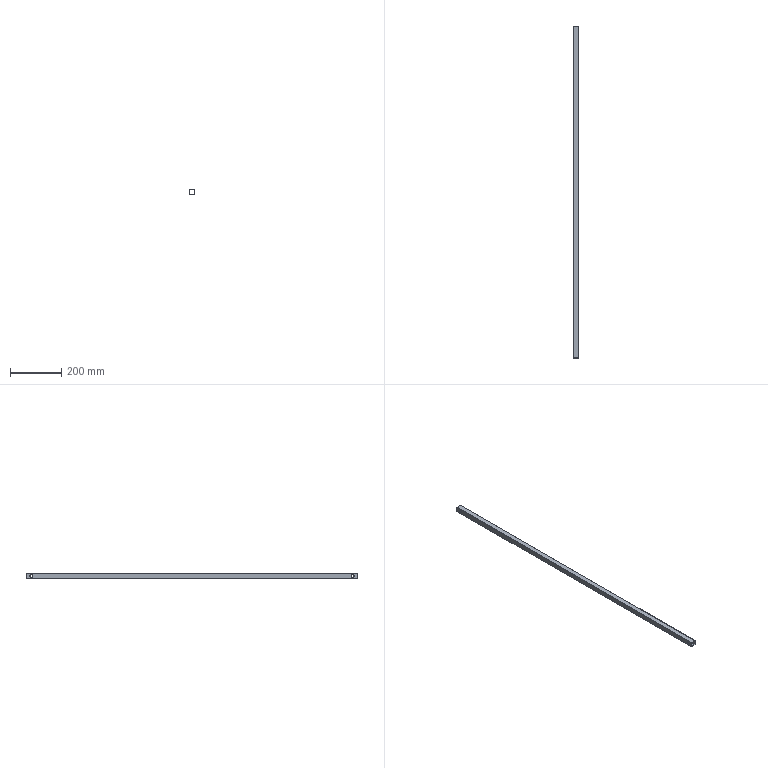Part | SolidWorks | features HoleWzd 1, WeldMemberFeat 1, WeldmentFeature 1 | 1 solid | 18 faces | box 20 x 1300 x 20 mm | volume 98454 mm3 | plane 10 | cylinder 8 | commonest cylinder face diameters 10.5 x8
STEP:
#1=CARTESIAN_POINT('',(-10.,20.,5.25));
#2=VERTEX_POINT('',#1);
#3=CARTESIAN_POINT('',(-10.,20.,-5.25));
#4=VERTEX_POINT('',#3);
#5=CARTESIAN_POINT('',(-10.,20.,0.));
#6=DIRECTION('',(1.,0.,0.));
#7=DIRECTION('',(0.,0.,-1.));
#8=AXIS2_PLACEMENT_3D('',#5,#6,#7);
#9=CIRCLE('',#8,5.25);
#10=EDGE_CURVE('',#2,#4,#9,.T.);
#11=ORIENTED_EDGE('',*,*,#10,.F.);
#12=CARTESIAN_POINT('',(-9.,20.,5.25));
#13=VERTEX_POINT('',#12);
#14=CARTESIAN_POINT('',(10.,20.,5.25));
#15=DIRECTION('',(1.,0.,0.));
#16=VECTOR('',#15,1000.);
#17=LINE('',#14,#16);
#18=EDGE_CURVE('',#2,#13,#17,.T.);
#19=ORIENTED_EDGE('',*,*,#18,.T.);
#20=CARTESIAN_POINT('',(-9.,20.,-5.25));
#21=VERTEX_POINT('',#20);
#22=CARTESIAN_POINT('',(-9.,20.,0.));
#23=DIRECTION('',(1.,0.,0.));
#24=DIRECTION('',(0.,0.,-1.));
#25=AXIS2_PLACEMENT_3D('',#22,#23,#24);
#26=CIRCLE('',#25,5.25);
#27=EDGE_CURVE('',#13,#21,#26,.T.);
#28=ORIENTED_EDGE('',*,*,#27,.T.);
#29=CARTESIAN_POINT('',(10.,20.,-5.25));
#30=DIRECTION('',(1.,0.,0.));
#31=VECTOR('',#30,1000.);
#32=LINE('',#29,#31);
#33=EDGE_CURVE('',#4,#21,#32,.T.);
#34=ORIENTED_EDGE('',*,*,#33,.F.);
#35=EDGE_LOOP('',(#11,#19,#28,#34));
#36=FACE_OUTER_BOUND('',#35,.T.);
#37=CARTESIAN_POINT('',(10.,20.,0.));
#38=DIRECTION('',(1.,0.,0.));
#39=DIRECTION('',(0.,0.,-1.));
#40=AXIS2_PLACEMENT_3D('',#37,#38,#39);
#41=CYLINDRICAL_SURFACE('',#40,5.25);
#42=ADVANCED_FACE('',(#36),#41,.F.);
#43=CARTESIAN_POINT('',(9.,20.,-5.25));
#44=VERTEX_POINT('',#43);
#45=CARTESIAN_POINT('',(9.,20.,5.25));
#46=VERTEX_POINT('',#45);
#47=CARTESIAN_POINT('',(9.,20.,0.));
#48=DIRECTION('',(-1.,0.,0.));
#49=DIRECTION('',(0.,0.,1.));
#50=AXIS2_PLACEMENT_3D('',#47,#48,#49);
#51=CIRCLE('',#50,5.25);
#52=EDGE_CURVE('',#44,#46,#51,.T.);
#53=ORIENTED_EDGE('',*,*,#52,.T.);
#54=CARTESIAN_POINT('',(10.,20.,5.25));
#55=VERTEX_POINT('',#54);
#56=CARTESIAN_POINT('',(10.,20.,5.25));
#57=DIRECTION('',(1.,0.,0.));
#58=VECTOR('',#57,1000.);
#59=LINE('',#56,#58);
#60=EDGE_CURVE('',#46,#55,#59,.T.);
#61=ORIENTED_EDGE('',*,*,#60,.T.);
#62=CARTESIAN_POINT('',(10.,20.,-5.25));
#63=VERTEX_POINT('',#62);
#64=CARTESIAN_POINT('',(10.,20.,0.));
#65=DIRECTION('',(1.,0.,0.));
#66=DIRECTION('',(0.,0.,-1.));
#67=AXIS2_PLACEMENT_3D('',#64,#65,#66);
#68=CIRCLE('',#67,5.25);
#69=EDGE_CURVE('',#55,#63,#68,.T.);
#70=ORIENTED_EDGE('',*,*,#69,.T.);
#71=CARTESIAN_POINT('',(10.,20.,-5.25));
#72=DIRECTION('',(1.,0.,0.));
#73=VECTOR('',#72,1000.);
#74=LINE('',#71,#73);
#75=EDGE_CURVE('',#44,#63,#74,.T.);
#76=ORIENTED_EDGE('',*,*,#75,.F.);
#77=EDGE_LOOP('',(#53,#61,#70,#76));
#78=FACE_OUTER_BOUND('',#77,.T.);
#79=CARTESIAN_POINT('',(10.,20.,0.));
#80=DIRECTION('',(1.,0.,0.));
#81=DIRECTION('',(0.,0.,-1.));
#82=AXIS2_PLACEMENT_3D('',#79,#80,#81);
#83=CYLINDRICAL_SURFACE('',#82,5.25);
#84=ADVANCED_FACE('',(#78),#83,.F.);
#85=CARTESIAN_POINT('',(9.,1280.,-5.25));
#86=VERTEX_POINT('',#85);
#87=CARTESIAN_POINT('',(9.,1280.,5.25));
#88=VERTEX_POINT('',#87);
#89=CARTESIAN_POINT('',(9.,1280.,0.));
#90=DIRECTION('',(-1.,0.,0.));
#91=DIRECTION('',(0.,0.,1.));
#92=AXIS2_PLACEMENT_3D('',#89,#90,#91);
#93=CIRCLE('',#92,5.25);
#94=EDGE_CURVE('',#86,#88,#93,.T.);
#95=ORIENTED_EDGE('',*,*,#94,.T.);
#96=CARTESIAN_POINT('',(10.,1280.,5.25));
#97=VERTEX_POINT('',#96);
#98=CARTESIAN_POINT('',(10.,1280.,5.25));
#99=DIRECTION('',(1.,0.,0.));
#100=VECTOR('',#99,1000.);
#101=LINE('',#98,#100);
#102=EDGE_CURVE('',#88,#97,#101,.T.);
#103=ORIENTED_EDGE('',*,*,#102,.T.);
#104=CARTESIAN_POINT('',(10.,1280.,-5.25));
#105=VERTEX_POINT('',#104);
#106=CARTESIAN_POINT('',(10.,1280.,0.));
#107=DIRECTION('',(1.,0.,0.));
#108=DIRECTION('',(0.,0.,-1.));
#109=AXIS2_PLACEMENT_3D('',#106,#107,#108);
#110=CIRCLE('',#109,5.25);
#111=EDGE_CURVE('',#97,#105,#110,.T.);
#112=ORIENTED_EDGE('',*,*,#111,.T.);
#113=CARTESIAN_POINT('',(10.,1280.,-5.25));
#114=DIRECTION('',(1.,0.,0.));
#115=VECTOR('',#114,1000.);
#116=LINE('',#113,#115);
#117=EDGE_CURVE('',#86,#105,#116,.T.);
#118=ORIENTED_EDGE('',*,*,#117,.F.);
#119=EDGE_LOOP('',(#95,#103,#112,#118));
#120=FACE_OUTER_BOUND('',#119,.T.);
#121=CARTESIAN_POINT('',(10.,1280.,0.));
#122=DIRECTION('',(1.,0.,0.));
#123=DIRECTION('',(0.,0.,-1.));
#124=AXIS2_PLACEMENT_3D('',#121,#122,#123);
#125=CYLINDRICAL_SURFACE('',#124,5.25);
#126=ADVANCED_FACE('',(#120),#125,.F.);
#127=CARTESIAN_POINT('',(-10.,1280.,5.25));
#128=VERTEX_POINT('',#127);
#129=CARTESIAN_POINT('',(-10.,1280.,-5.25));
#130=VERTEX_POINT('',#129);
#131=CARTESIAN_POINT('',(-10.,1280.,0.));
#132=DIRECTION('',(1.,0.,0.));
#133=DIRECTION('',(0.,0.,-1.));
#134=AXIS2_PLACEMENT_3D('',#131,#132,#133);
#135=CIRCLE('',#134,5.25);
#136=EDGE_CURVE('',#128,#130,#135,.T.);
#137=ORIENTED_EDGE('',*,*,#136,.F.);
#138=CARTESIAN_POINT('',(-9.,1280.,5.25));
#139=VERTEX_POINT('',#138);
#140=CARTESIAN_POINT('',(10.,1280.,5.25));
#141=DIRECTION('',(1.,0.,0.));
#142=VECTOR('',#141,1000.);
#143=LINE('',#140,#142);
#144=EDGE_CURVE('',#128,#139,#143,.T.);
#145=ORIENTED_EDGE('',*,*,#144,.T.);
#146=CARTESIAN_POINT('',(-9.,1280.,-5.25));
#147=VERTEX_POINT('',#146);
#148=CARTESIAN_POINT('',(-9.,1280.,0.));
#149=DIRECTION('',(1.,0.,0.));
#150=DIRECTION('',(0.,0.,-1.));
#151=AXIS2_PLACEMENT_3D('',#148,#149,#150);
#152=CIRCLE('',#151,5.25);
#153=EDGE_CURVE('',#139,#147,#152,.T.);
#154=ORIENTED_EDGE('',*,*,#153,.T.);
#155=CARTESIAN_POINT('',(10.,1280.,-5.25));
#156=DIRECTION('',(1.,0.,0.));
#157=VECTOR('',#156,1000.);
#158=LINE('',#155,#157);
#159=EDGE_CURVE('',#130,#147,#158,.T.);
#160=ORIENTED_EDGE('',*,*,#159,.F.);
#161=EDGE_LOOP('',(#137,#145,#154,#160));
#162=FACE_OUTER_BOUND('',#161,.T.);
#163=CARTESIAN_POINT('',(10.,1280.,0.));
#164=DIRECTION('',(1.,0.,0.));
#165=DIRECTION('',(0.,0.,-1.));
#166=AXIS2_PLACEMENT_3D('',#163,#164,#165);
#167=CYLINDRICAL_SURFACE('',#166,5.25);
#168=ADVANCED_FACE('',(#162),#167,.F.);
#169=CARTESIAN_POINT('',(-9.,0.,9.));
#170=VERTEX_POINT('',#169);
#171=CARTESIAN_POINT('',(9.,0.,9.));
#172=VERTEX_POINT('',#171);
#173=CARTESIAN_POINT('',(-9.,0.,9.));
#174=DIRECTION('',(1.,0.,0.));
#175=VECTOR('',#174,1000.);
#176=LINE('',#173,#175);
#177=EDGE_CURVE('',#170,#172,#176,.T.);
#178=ORIENTED_EDGE('',*,*,#177,.F.);
#179=CARTESIAN_POINT('',(-9.,1300.,9.));
#180=VERTEX_POINT('',#179);
#181=CARTESIAN_POINT('',(-9.,1300.,9.));
#182=DIRECTION('',(0.,-1.,0.));
#183=VECTOR('',#182,1000.);
#184=LINE('',#181,#183);
#185=EDGE_CURVE('',#180,#170,#184,.T.);
#186=ORIENTED_EDGE('',*,*,#185,.F.);
#187=CARTESIAN_POINT('',(9.,1300.,9.));
#188=VERTEX_POINT('',#187);
#189=CARTESIAN_POINT('',(-9.,1300.,9.));
#190=DIRECTION('',(1.,0.,0.));
#191=VECTOR('',#190,1000.);
#192=LINE('',#189,#191);
#193=EDGE_CURVE('',#180,#188,#192,.T.);
#194=ORIENTED_EDGE('',*,*,#193,.T.);
#195=CARTESIAN_POINT('',(9.,1300.,9.));
#196=DIRECTION('',(0.,-1.,0.));
#197=VECTOR('',#196,1000.);
#198=LINE('',#195,#197);
#199=EDGE_CURVE('',#188,#172,#198,.T.);
#200=ORIENTED_EDGE('',*,*,#199,.T.);
#201=EDGE_LOOP('',(#178,#186,#194,#200));
#202=FACE_OUTER_BOUND('',#201,.T.);
#203=CARTESIAN_POINT('',(-9.,1300.,9.));
#204=DIRECTION('',(0.,0.,-1.));
#205=DIRECTION('',(-1.,0.,0.));
#206=AXIS2_PLACEMENT_3D('',#203,#204,#205);
#207=PLANE('',#206);
#208=ADVANCED_FACE('',(#202),#207,.T.);
#209=CARTESIAN_POINT('',(-9.,20.,0.));
#210=DIRECTION('',(1.,0.,0.));
#211=DIRECTION('',(0.,0.,-1.));
#212=AXIS2_PLACEMENT_3D('',#209,#210,#211);
#213=CIRCLE('',#212,5.25);
#214=EDGE_CURVE('',#21,#13,#213,.T.);
#215=ORIENTED_EDGE('',*,*,#214,.F.);
#216=ORIENTED_EDGE('',*,*,#27,.F.);
#217=EDGE_LOOP('',(#215,#216));
#218=FACE_BOUND('',#217,.T.);
#219=CARTESIAN_POINT('',(-9.,1280.,0.));
#220=DIRECTION('',(1.,0.,0.));
#221=DIRECTION('',(0.,0.,-1.));
#222=AXIS2_PLACEMENT_3D('',#219,#220,#221);
#223=CIRCLE('',#222,5.25);
#224=EDGE_CURVE('',#147,#139,#223,.T.);
#225=ORIENTED_EDGE('',*,*,#224,.F.);
#226=ORIENTED_EDGE('',*,*,#153,.F.);
#227=EDGE_LOOP('',(#225,#226));
#228=FACE_BOUND('',#227,.T.);
#229=CARTESIAN_POINT('',(-9.,0.,-9.));
#230=VERTEX_POINT('',#229);
#231=CARTESIAN_POINT('',(-9.,0.,-9.));
#232=DIRECTION('',(0.,0.,1.));
#233=VECTOR('',#232,1000.);
#234=LINE('',#231,#233);
#235=EDGE_CURVE('',#230,#170,#234,.T.);
#236=ORIENTED_EDGE('',*,*,#235,.F.);
#237=CARTESIAN_POINT('',(-9.,1300.,-9.));
#238=VERTEX_POINT('',#237);
#239=CARTESIAN_POINT('',(-9.,1300.,-9.));
#240=DIRECTION('',(0.,-1.,0.));
#241=VECTOR('',#240,1000.);
#242=LINE('',#239,#241);
#243=EDGE_CURVE('',#238,#230,#242,.T.);
#244=ORIENTED_EDGE('',*,*,#243,.F.);
#245=CARTESIAN_POINT('',(-9.,1300.,-9.));
#246=DIRECTION('',(0.,0.,1.));
#247=VECTOR('',#246,1000.);
#248=LINE('',#245,#247);
#249=EDGE_CURVE('',#238,#180,#248,.T.);
#250=ORIENTED_EDGE('',*,*,#249,.T.);
#251=ORIENTED_EDGE('',*,*,#185,.T.);
#252=EDGE_LOOP('',(#236,#244,#250,#251));
#253=FACE_OUTER_BOUND('',#252,.T.);
#254=CARTESIAN_POINT('',(-9.,1300.,-9.));
#255=DIRECTION('',(1.,0.,0.));
#256=DIRECTION('',(0.,0.,-1.));
#257=AXIS2_PLACEMENT_3D('',#254,#255,#256);
#258=PLANE('',#257);
#259=ADVANCED_FACE('',(#218,#228,#253),#258,.T.);
#260=CARTESIAN_POINT('',(9.,0.,-9.));
#261=VERTEX_POINT('',#260);
#262=CARTESIAN_POINT('',(-9.,0.,-9.));
#263=DIRECTION('',(-1.,0.,0.));
#264=VECTOR('',#263,1000.);
#265=LINE('',#262,#264);
#266=EDGE_CURVE('',#261,#230,#265,.T.);
#267=ORIENTED_EDGE('',*,*,#266,.F.);
#268=CARTESIAN_POINT('',(9.,1300.,-9.));
#269=VERTEX_POINT('',#268);
#270=CARTESIAN_POINT('',(9.,1300.,-9.));
#271=DIRECTION('',(0.,-1.,0.));
#272=VECTOR('',#271,1000.);
#273=LINE('',#270,#272);
#274=EDGE_CURVE('',#269,#261,#273,.T.);
#275=ORIENTED_EDGE('',*,*,#274,.F.);
#276=CARTESIAN_POINT('',(-9.,1300.,-9.));
#277=DIRECTION('',(-1.,0.,0.));
#278=VECTOR('',#277,1000.);
#279=LINE('',#276,#278);
#280=EDGE_CURVE('',#269,#238,#279,.T.);
#281=ORIENTED_EDGE('',*,*,#280,.T.);
#282=ORIENTED_EDGE('',*,*,#243,.T.);
#283=EDGE_LOOP('',(#267,#275,#281,#282));
#284=FACE_OUTER_BOUND('',#283,.T.);
#285=CARTESIAN_POINT('',(-9.,1300.,-9.));
#286=DIRECTION('',(0.,0.,1.));
#287=DIRECTION('',(1.,0.,0.));
#288=AXIS2_PLACEMENT_3D('',#285,#286,#287);
#289=PLANE('',#288);
#290=ADVANCED_FACE('',(#284),#289,.T.);
#291=CARTESIAN_POINT('',(-10.,0.,10.));
#292=VERTEX_POINT('',#291);
#293=CARTESIAN_POINT('',(10.,0.,10.));
#294=VERTEX_POINT('',#293);
#295=CARTESIAN_POINT('',(-10.,0.,10.));
#296=DIRECTION('',(1.,0.,0.));
#297=VECTOR('',#296,1000.);
#298=LINE('',#295,#297);
#299=EDGE_CURVE('',#292,#294,#298,.T.);
#300=ORIENTED_EDGE('',*,*,#299,.T.);
#301=CARTESIAN_POINT('',(10.,1300.,10.));
#302=VERTEX_POINT('',#301);
#303=CARTESIAN_POINT('',(10.,1300.,10.));
#304=DIRECTION('',(0.,-1.,0.));
#305=VECTOR('',#304,1000.);
#306=LINE('',#303,#305);
#307=EDGE_CURVE('',#302,#294,#306,.T.);
#308=ORIENTED_EDGE('',*,*,#307,.F.);
#309=CARTESIAN_POINT('',(-10.,1300.,10.));
#310=VERTEX_POINT('',#309);
#311=CARTESIAN_POINT('',(-10.,1300.,10.));
#312=DIRECTION('',(1.,0.,0.));
#313=VECTOR('',#312,1000.);
#314=LINE('',#311,#313);
#315=EDGE_CURVE('',#310,#302,#314,.T.);
#316=ORIENTED_EDGE('',*,*,#315,.F.);
#317=CARTESIAN_POINT('',(-10.,1300.,10.));
#318=DIRECTION('',(0.,-1.,0.));
#319=VECTOR('',#318,1000.);
#320=LINE('',#317,#319);
#321=EDGE_CURVE('',#310,#292,#320,.T.);
#322=ORIENTED_EDGE('',*,*,#321,.T.);
#323=EDGE_LOOP('',(#300,#308,#316,#322));
#324=FACE_OUTER_BOUND('',#323,.T.);
#325=CARTESIAN_POINT('',(-10.,1300.,10.));
#326=DIRECTION('',(0.,0.,-1.));
#327=DIRECTION('',(-1.,0.,0.));
#328=AXIS2_PLACEMENT_3D('',#325,#326,#327);
#329=PLANE('',#328);
#330=ADVANCED_FACE('',(#324),#329,.F.);
#331=CARTESIAN_POINT('',(10.,20.,0.));
#332=DIRECTION('',(1.,0.,0.));
#333=DIRECTION('',(0.,0.,-1.));
#334=AXIS2_PLACEMENT_3D('',#331,#332,#333);
#335=CIRCLE('',#334,5.25);
#336=EDGE_CURVE('',#63,#55,#335,.T.);
#337=ORIENTED_EDGE('',*,*,#336,.F.);
#338=ORIENTED_EDGE('',*,*,#69,.F.);
#339=EDGE_LOOP('',(#337,#338));
#340=FACE_BOUND('',#339,.T.);
#341=CARTESIAN_POINT('',(10.,1280.,0.));
#342=DIRECTION('',(1.,0.,0.));
#343=DIRECTION('',(0.,0.,-1.));
#344=AXIS2_PLACEMENT_3D('',#341,#342,#343);
#345=CIRCLE('',#344,5.25);
#346=EDGE_CURVE('',#105,#97,#345,.T.);
#347=ORIENTED_EDGE('',*,*,#346,.F.);
#348=ORIENTED_EDGE('',*,*,#111,.F.);
#349=EDGE_LOOP('',(#347,#348));
#350=FACE_BOUND('',#349,.T.);
#351=CARTESIAN_POINT('',(10.,0.,-10.));
#352=VERTEX_POINT('',#351);
#353=CARTESIAN_POINT('',(10.,0.,-10.));
#354=DIRECTION('',(0.,0.,-1.));
#355=VECTOR('',#354,1000.);
#356=LINE('',#353,#355);
#357=EDGE_CURVE('',#294,#352,#356,.T.);
#358=ORIENTED_EDGE('',*,*,#357,.T.);
#359=CARTESIAN_POINT('',(10.,1300.,-10.));
#360=VERTEX_POINT('',#359);
#361=CARTESIAN_POINT('',(10.,1300.,-10.));
#362=DIRECTION('',(0.,-1.,0.));
#363=VECTOR('',#362,1000.);
#364=LINE('',#361,#363);
#365=EDGE_CURVE('',#360,#352,#364,.T.);
#366=ORIENTED_EDGE('',*,*,#365,.F.);
#367=CARTESIAN_POINT('',(10.,1300.,-10.));
#368=DIRECTION('',(0.,0.,-1.));
#369=VECTOR('',#368,1000.);
#370=LINE('',#367,#369);
#371=EDGE_CURVE('',#302,#360,#370,.T.);
#372=ORIENTED_EDGE('',*,*,#371,.F.);
#373=ORIENTED_EDGE('',*,*,#307,.T.);
#374=EDGE_LOOP('',(#358,#366,#372,#373));
#375=FACE_OUTER_BOUND('',#374,.T.);
#376=CARTESIAN_POINT('',(10.,1300.,-10.));
#377=DIRECTION('',(-1.,0.,0.));
#378=DIRECTION('',(0.,0.,1.));
#379=AXIS2_PLACEMENT_3D('',#376,#377,#378);
#380=PLANE('',#379);
#381=ADVANCED_FACE('',(#340,#350,#375),#380,.F.);
#382=CARTESIAN_POINT('',(-10.,0.,-10.));
#383=VERTEX_POINT('',#382);
#384=CARTESIAN_POINT('',(-10.,0.,-10.));
#385=DIRECTION('',(-1.,0.,0.));
#386=VECTOR('',#385,1000.);
#387=LINE('',#384,#386);
#388=EDGE_CURVE('',#352,#383,#387,.T.);
#389=ORIENTED_EDGE('',*,*,#388,.T.);
#390=CARTESIAN_POINT('',(-10.,1300.,-10.));
#391=VERTEX_POINT('',#390);
#392=CARTESIAN_POINT('',(-10.,1300.,-10.));
#393=DIRECTION('',(0.,-1.,0.));
#394=VECTOR('',#393,1000.);
#395=LINE('',#392,#394);
#396=EDGE_CURVE('',#391,#383,#395,.T.);
#397=ORIENTED_EDGE('',*,*,#396,.F.);
#398=CARTESIAN_POINT('',(-10.,1300.,-10.));
#399=DIRECTION('',(-1.,0.,0.));
#400=VECTOR('',#399,1000.);
#401=LINE('',#398,#400);
#402=EDGE_CURVE('',#360,#391,#401,.T.);
#403=ORIENTED_EDGE('',*,*,#402,.F.);
#404=ORIENTED_EDGE('',*,*,#365,.T.);
#405=EDGE_LOOP('',(#389,#397,#403,#404));
#406=FACE_OUTER_BOUND('',#405,.T.);
#407=CARTESIAN_POINT('',(-10.,1300.,-10.));
#408=DIRECTION('',(0.,0.,1.));
#409=DIRECTION('',(1.,0.,0.));
#410=AXIS2_PLACEMENT_3D('',#407,#408,#409);
#411=PLANE('',#410);
#412=ADVANCED_FACE('',(#406),#411,.F.);
#413=CARTESIAN_POINT('',(-10.,20.,0.));
#414=DIRECTION('',(1.,0.,0.));
#415=DIRECTION('',(0.,0.,-1.));
#416=AXIS2_PLACEMENT_3D('',#413,#414,#415);
#417=CIRCLE('',#416,5.25);
#418=EDGE_CURVE('',#4,#2,#417,.T.);
#419=ORIENTED_EDGE('',*,*,#418,.T.);
#420=ORIENTED_EDGE('',*,*,#10,.T.);
#421=EDGE_LOOP('',(#419,#420));
#422=FACE_BOUND('',#421,.T.);
#423=CARTESIAN_POINT('',(-10.,1280.,0.));
#424=DIRECTION('',(1.,0.,0.));
#425=DIRECTION('',(0.,0.,-1.));
#426=AXIS2_PLACEMENT_3D('',#423,#424,#425);
#427=CIRCLE('',#426,5.25);
#428=EDGE_CURVE('',#130,#128,#427,.T.);
#429=ORIENTED_EDGE('',*,*,#428,.T.);
#430=ORIENTED_EDGE('',*,*,#136,.T.);
#431=EDGE_LOOP('',(#429,#430));
#432=FACE_BOUND('',#431,.T.);
#433=CARTESIAN_POINT('',(-10.,0.,-10.));
#434=DIRECTION('',(0.,0.,1.));
#435=VECTOR('',#434,1000.);
#436=LINE('',#433,#435);
#437=EDGE_CURVE('',#383,#292,#436,.T.);
#438=ORIENTED_EDGE('',*,*,#437,.T.);
#439=ORIENTED_EDGE('',*,*,#321,.F.);
#440=CARTESIAN_POINT('',(-10.,1300.,-10.));
#441=DIRECTION('',(0.,0.,1.));
#442=VECTOR('',#441,1000.);
#443=LINE('',#440,#442);
#444=EDGE_CURVE('',#391,#310,#443,.T.);
#445=ORIENTED_EDGE('',*,*,#444,.F.);
#446=ORIENTED_EDGE('',*,*,#396,.T.);
#447=EDGE_LOOP('',(#438,#439,#445,#446));
#448=FACE_OUTER_BOUND('',#447,.T.);
#449=CARTESIAN_POINT('',(-10.,1300.,-10.));
#450=DIRECTION('',(1.,0.,0.));
#451=DIRECTION('',(0.,0.,-1.));
#452=AXIS2_PLACEMENT_3D('',#449,#450,#451);
#453=PLANE('',#452);
#454=ADVANCED_FACE('',(#422,#432,#448),#453,.F.);
#455=ORIENTED_EDGE('',*,*,#52,.F.);
#456=CARTESIAN_POINT('',(9.,20.,0.));
#457=DIRECTION('',(-1.,0.,0.));
#458=DIRECTION('',(0.,0.,1.));
#459=AXIS2_PLACEMENT_3D('',#456,#457,#458);
#460=CIRCLE('',#459,5.25);
#461=EDGE_CURVE('',#46,#44,#460,.T.);
#462=ORIENTED_EDGE('',*,*,#461,.F.);
#463=EDGE_LOOP('',(#455,#462));
#464=FACE_BOUND('',#463,.T.);
#465=ORIENTED_EDGE('',*,*,#94,.F.);
#466=CARTESIAN_POINT('',(9.,1280.,0.));
#467=DIRECTION('',(-1.,0.,0.));
#468=DIRECTION('',(0.,0.,1.));
#469=AXIS2_PLACEMENT_3D('',#466,#467,#468);
#470=CIRCLE('',#469,5.25);
#471=EDGE_CURVE('',#88,#86,#470,.T.);
#472=ORIENTED_EDGE('',*,*,#471,.F.);
#473=EDGE_LOOP('',(#465,#472));
#474=FACE_BOUND('',#473,.T.);
#475=CARTESIAN_POINT('',(9.,0.,-9.));
#476=DIRECTION('',(0.,0.,-1.));
#477=VECTOR('',#476,1000.);
#478=LINE('',#475,#477);
#479=EDGE_CURVE('',#172,#261,#478,.T.);
#480=ORIENTED_EDGE('',*,*,#479,.F.);
#481=ORIENTED_EDGE('',*,*,#199,.F.);
#482=CARTESIAN_POINT('',(9.,1300.,-9.));
#483=DIRECTION('',(0.,0.,-1.));
#484=VECTOR('',#483,1000.);
#485=LINE('',#482,#484);
#486=EDGE_CURVE('',#188,#269,#485,.T.);
#487=ORIENTED_EDGE('',*,*,#486,.T.);
#488=ORIENTED_EDGE('',*,*,#274,.T.);
#489=EDGE_LOOP('',(#480,#481,#487,#488));
#490=FACE_OUTER_BOUND('',#489,.T.);
#491=CARTESIAN_POINT('',(9.,1300.,-9.));
#492=DIRECTION('',(-1.,0.,0.));
#493=DIRECTION('',(0.,0.,1.));
#494=AXIS2_PLACEMENT_3D('',#491,#492,#493);
#495=PLANE('',#494);
#496=ADVANCED_FACE('',(#464,#474,#490),#495,.T.);
#497=ORIENTED_EDGE('',*,*,#315,.T.);
#498=ORIENTED_EDGE('',*,*,#371,.T.);
#499=ORIENTED_EDGE('',*,*,#402,.T.);
#500=ORIENTED_EDGE('',*,*,#444,.T.);
#501=EDGE_LOOP('',(#497,#498,#499,#500));
#502=FACE_OUTER_BOUND('',#501,.T.);
#503=ORIENTED_EDGE('',*,*,#193,.F.);
#504=ORIENTED_EDGE('',*,*,#249,.F.);
#505=ORIENTED_EDGE('',*,*,#280,.F.);
#506=ORIENTED_EDGE('',*,*,#486,.F.);
#507=EDGE_LOOP('',(#503,#504,#505,#506));
#508=FACE_BOUND('',#507,.T.);
#509=CARTESIAN_POINT('',(0.,1300.,0.));
#510=DIRECTION('',(0.,-1.,0.));
#511=DIRECTION('',(0.,0.,-1.));
#512=AXIS2_PLACEMENT_3D('',#509,#510,#511);
#513=PLANE('',#512);
#514=ADVANCED_FACE('',(#502,#508),#513,.F.);
#515=ORIENTED_EDGE('',*,*,#299,.F.);
#516=ORIENTED_EDGE('',*,*,#437,.F.);
#517=ORIENTED_EDGE('',*,*,#388,.F.);
#518=ORIENTED_EDGE('',*,*,#357,.F.);
#519=EDGE_LOOP('',(#515,#516,#517,#518));
#520=FACE_OUTER_BOUND('',#519,.T.);
#521=ORIENTED_EDGE('',*,*,#177,.T.);
#522=ORIENTED_EDGE('',*,*,#479,.T.);
#523=ORIENTED_EDGE('',*,*,#266,.T.);
#524=ORIENTED_EDGE('',*,*,#235,.T.);
#525=EDGE_LOOP('',(#521,#522,#523,#524));
#526=FACE_BOUND('',#525,.T.);
#527=CARTESIAN_POINT('',(0.,0.,0.));
#528=DIRECTION('',(0.,-1.,0.));
#529=DIRECTION('',(0.,0.,-1.));
#530=AXIS2_PLACEMENT_3D('',#527,#528,#529);
#531=PLANE('',#530);
#532=ADVANCED_FACE('',(#520,#526),#531,.T.);
#533=ORIENTED_EDGE('',*,*,#144,.F.);
#534=ORIENTED_EDGE('',*,*,#428,.F.);
#535=ORIENTED_EDGE('',*,*,#159,.T.);
#536=ORIENTED_EDGE('',*,*,#224,.T.);
#537=EDGE_LOOP('',(#533,#534,#535,#536));
#538=FACE_OUTER_BOUND('',#537,.T.);
#539=CARTESIAN_POINT('',(10.,1280.,0.));
#540=DIRECTION('',(1.,0.,0.));
#541=DIRECTION('',(0.,0.,-1.));
#542=AXIS2_PLACEMENT_3D('',#539,#540,#541);
#543=CYLINDRICAL_SURFACE('',#542,5.25);
#544=ADVANCED_FACE('',(#538),#543,.F.);
#545=ORIENTED_EDGE('',*,*,#102,.F.);
#546=ORIENTED_EDGE('',*,*,#471,.T.);
#547=ORIENTED_EDGE('',*,*,#117,.T.);
#548=ORIENTED_EDGE('',*,*,#346,.T.);
#549=EDGE_LOOP('',(#545,#546,#547,#548));
#550=FACE_OUTER_BOUND('',#549,.T.);
#551=CARTESIAN_POINT('',(10.,1280.,0.));
#552=DIRECTION('',(1.,0.,0.));
#553=DIRECTION('',(0.,0.,-1.));
#554=AXIS2_PLACEMENT_3D('',#551,#552,#553);
#555=CYLINDRICAL_SURFACE('',#554,5.25);
#556=ADVANCED_FACE('',(#550),#555,.F.);
#557=ORIENTED_EDGE('',*,*,#60,.F.);
#558=ORIENTED_EDGE('',*,*,#461,.T.);
#559=ORIENTED_EDGE('',*,*,#75,.T.);
#560=ORIENTED_EDGE('',*,*,#336,.T.);
#561=EDGE_LOOP('',(#557,#558,#559,#560));
#562=FACE_OUTER_BOUND('',#561,.T.);
#563=CARTESIAN_POINT('',(10.,20.,0.));
#564=DIRECTION('',(1.,0.,0.));
#565=DIRECTION('',(0.,0.,-1.));
#566=AXIS2_PLACEMENT_3D('',#563,#564,#565);
#567=CYLINDRICAL_SURFACE('',#566,5.25);
#568=ADVANCED_FACE('',(#562),#567,.F.);
#569=ORIENTED_EDGE('',*,*,#18,.F.);
#570=ORIENTED_EDGE('',*,*,#418,.F.);
#571=ORIENTED_EDGE('',*,*,#33,.T.);
#572=ORIENTED_EDGE('',*,*,#214,.T.);
#573=EDGE_LOOP('',(#569,#570,#571,#572));
#574=FACE_OUTER_BOUND('',#573,.T.);
#575=CARTESIAN_POINT('',(10.,20.,0.));
#576=DIRECTION('',(1.,0.,0.));
#577=DIRECTION('',(0.,0.,-1.));
#578=AXIS2_PLACEMENT_3D('',#575,#576,#577);
#579=CYLINDRICAL_SURFACE('',#578,5.25);
#580=ADVANCED_FACE('',(#574),#579,.F.);
#581=CLOSED_SHELL('',(#42,#84,#126,#168,#208,#259,#290,#330,#381,#412,#454,#496,#514,#532,#544,#556,#568,#580));
#582=MANIFOLD_SOLID_BREP('',#581);
#583=CARTESIAN_POINT('',(0.,0.,0.));
#584=DIRECTION('',(0.,0.,1.));
#585=DIRECTION('',(1.,0.,0.));
#586=AXIS2_PLACEMENT_3D('',#583,#584,#585);
#587=(LENGTH_UNIT()NAMED_UNIT(*)SI_UNIT(.MILLI.,.METRE.));
#588=UNCERTAINTY_MEASURE_WITH_UNIT(LENGTH_MEASURE(0.00001),#587,'','');
#589=(NAMED_UNIT(*)PLANE_ANGLE_UNIT()SI_UNIT($,.RADIAN.));
#590=(NAMED_UNIT(*)SI_UNIT($,.STERADIAN.)SOLID_ANGLE_UNIT());
#591=(GEOMETRIC_REPRESENTATION_CONTEXT(3)GLOBAL_UNCERTAINTY_ASSIGNED_CONTEXT((#588))GLOBAL_UNIT_ASSIGNED_CONTEXT((#587,#589,#590))REPRESENTATION_CONTEXT('',''));
#592=ADVANCED_BREP_SHAPE_REPRESENTATION('',(#582,#586),#591);